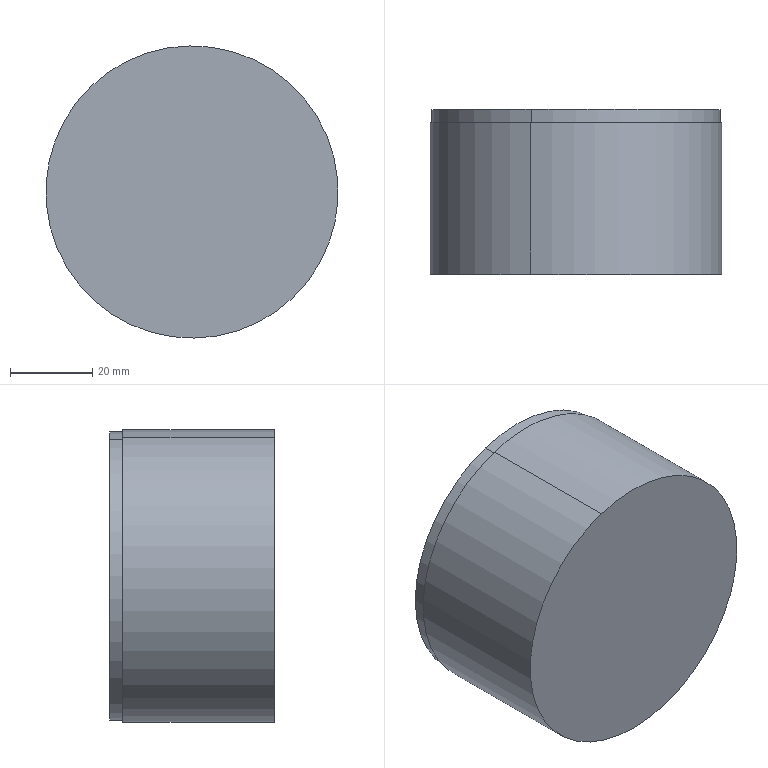Part | NX | features BREP 1 | 1 solid | 304 faces | box 71 x 40 x 71 mm | volume 141415 mm3 | cylinder 168 | spline 78 | cone 36 | plane 22 | commonest cylinder face diameters 5 x122 8 x28 10 x6 26 x3 66 x3 19 x2